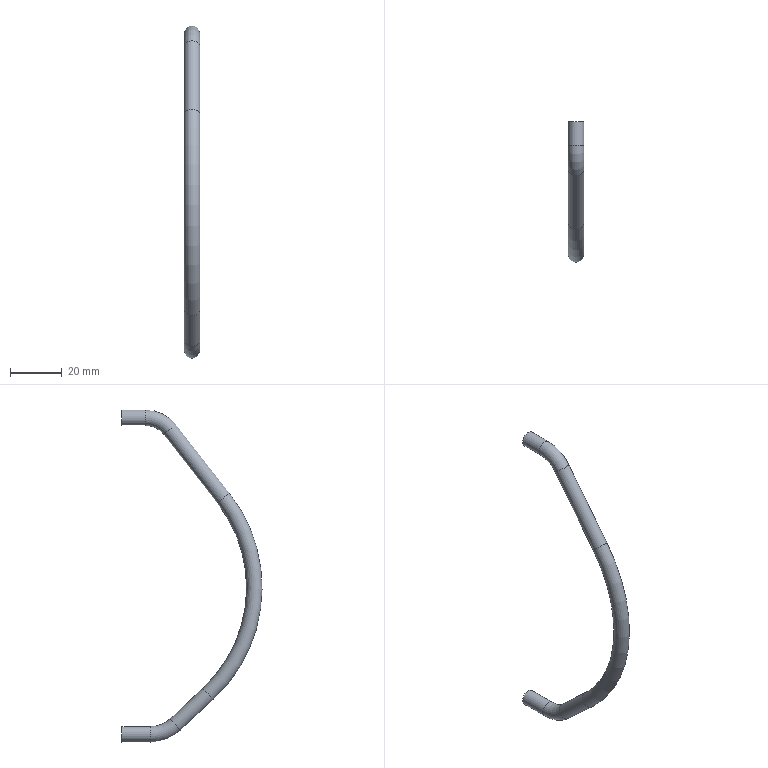Part | STEP file | 1-70.3 | 1 solid | 16 faces | box 6 x 54 x 128 mm | volume 1514 mm3 | cylinder 8 | torus 6 | plane 2 | commonest cylinder face diameters 5 x4 6 x4
STEP:
#1=CARTESIAN_POINT('',(0.,0.,0.));
#2=DIRECTION('',(0.,0.,1.));
#3=DIRECTION('',(1.,0.,0.));
#4=AXIS2_PLACEMENT_3D('',#1,#2,#3);
#5=CARTESIAN_POINT('',(-3.,0.,0.));
#6=VERTEX_POINT('',#5);
#7=CARTESIAN_POINT('',(0.,0.,0.));
#8=DIRECTION('',(0.,1.,0.));
#9=DIRECTION('',(-1.,0.,0.));
#10=AXIS2_PLACEMENT_3D('',#7,#8,#9);
#11=CIRCLE('',#10,3.);
#12=CARTESIAN_POINT('',(0.,0.,0.));
#13=DIRECTION('',(0.,-1.,0.));
#14=DIRECTION('',(-1.,0.,0.));
#15=AXIS2_PLACEMENT_3D('',#12,#13,#14);
#16=CYLINDRICAL_SURFACE('',#15,3.);
#17=CARTESIAN_POINT('',(6.283,0.));
#18=DIRECTION('',(-1.,0.));
#19=VECTOR('',#18,1.);
#20=LINE('',#17,#19);
#21=(GEOMETRIC_REPRESENTATION_CONTEXT(2)PARAMETRIC_REPRESENTATION_CONTEXT()REPRESENTATION_CONTEXT('',''));
#22=DEFINITIONAL_REPRESENTATION('',(#20),#21);
#23=PCURVE('',#16,#22);
#24=CARTESIAN_POINT('',(0.,0.,0.));
#25=DIRECTION('',(0.,1.,0.));
#26=DIRECTION('',(1.,0.,0.));
#27=AXIS2_PLACEMENT_3D('',#24,#25,#26);
#28=PLANE('',#27);
#29=CARTESIAN_POINT('',(0.,0.));
#30=DIRECTION('',(-1.,0.));
#31=AXIS2_PLACEMENT_2D('',#29,#30);
#32=CIRCLE('',#31,3.);
#33=(GEOMETRIC_REPRESENTATION_CONTEXT(2)PARAMETRIC_REPRESENTATION_CONTEXT()REPRESENTATION_CONTEXT('',''));
#34=DEFINITIONAL_REPRESENTATION('',(#32),#33);
#35=PCURVE('',#28,#34);
#36=SURFACE_CURVE('',#11,(#23,#35),.PCURVE_S1.);
#37=EDGE_CURVE('',#6,#6,#36,.T.);
#38=ORIENTED_EDGE('',*,*,#37,.F.);
#39=CARTESIAN_POINT('',(-3.,-9.,0.));
#40=VERTEX_POINT('',#39);
#41=CARTESIAN_POINT('',(-3.,0.,0.));
#42=DIRECTION('',(0.,-1.,0.));
#43=VECTOR('',#42,1.);
#44=LINE('',#41,#43);
#45=CARTESIAN_POINT('',(6.283,0.));
#46=DIRECTION('',(0.,1.));
#47=VECTOR('',#46,1.);
#48=LINE('',#45,#47);
#49=(GEOMETRIC_REPRESENTATION_CONTEXT(2)PARAMETRIC_REPRESENTATION_CONTEXT()REPRESENTATION_CONTEXT('',''));
#50=DEFINITIONAL_REPRESENTATION('',(#48),#49);
#51=PCURVE('',#16,#50);
#52=CARTESIAN_POINT('',(0.,0.));
#53=DIRECTION('',(0.,1.));
#54=VECTOR('',#53,1.);
#55=LINE('',#52,#54);
#56=(GEOMETRIC_REPRESENTATION_CONTEXT(2)PARAMETRIC_REPRESENTATION_CONTEXT()REPRESENTATION_CONTEXT('',''));
#57=DEFINITIONAL_REPRESENTATION('',(#55),#56);
#58=PCURVE('',#16,#57);
#59=SEAM_CURVE('',#44,(#51,#58),.PCURVE_S1.);
#60=EDGE_CURVE('',#6,#40,#59,.T.);
#61=ORIENTED_EDGE('',*,*,#60,.T.);
#62=CARTESIAN_POINT('',(0.,-9.,0.));
#63=DIRECTION('',(0.,-1.,0.));
#64=DIRECTION('',(-1.,0.,0.));
#65=AXIS2_PLACEMENT_3D('',#62,#63,#64);
#66=CIRCLE('',#65,3.);
#67=CARTESIAN_POINT('',(0.,9.));
#68=DIRECTION('',(1.,0.));
#69=VECTOR('',#68,1.);
#70=LINE('',#67,#69);
#71=(GEOMETRIC_REPRESENTATION_CONTEXT(2)PARAMETRIC_REPRESENTATION_CONTEXT()REPRESENTATION_CONTEXT('',''));
#72=DEFINITIONAL_REPRESENTATION('',(#70),#71);
#73=PCURVE('',#16,#72);
#74=CARTESIAN_POINT('',(0.,-9.,-12.));
#75=DIRECTION('',(-1.,0.,0.));
#76=DIRECTION('',(0.,0.,1.));
#77=AXIS2_PLACEMENT_3D('',#74,#75,#76);
#78=TOROIDAL_SURFACE('',#77,12.,3.);
#79=CARTESIAN_POINT('',(6.283,1.571));
#80=DIRECTION('',(0.,1.));
#81=VECTOR('',#80,1.);
#82=LINE('',#79,#81);
#83=(GEOMETRIC_REPRESENTATION_CONTEXT(2)PARAMETRIC_REPRESENTATION_CONTEXT()REPRESENTATION_CONTEXT('',''));
#84=DEFINITIONAL_REPRESENTATION('',(#82),#83);
#85=PCURVE('',#78,#84);
#86=SURFACE_CURVE('',#66,(#73,#85),.PCURVE_S1.);
#87=EDGE_CURVE('',#40,#40,#86,.T.);
#88=ORIENTED_EDGE('',*,*,#87,.F.);
#89=ORIENTED_EDGE('',*,*,#60,.F.);
#90=EDGE_LOOP('',(#38,#61,#88,#89));
#91=FACE_BOUND('',#90,.T.);
#92=ADVANCED_FACE('',(#91),#16,.T.);
#93=ORIENTED_EDGE('',*,*,#87,.T.);
#94=CARTESIAN_POINT('',(-3.,-18.45,-4.604));
#95=VERTEX_POINT('',#94);
#96=CARTESIAN_POINT('',(-3.,-9.,-12.));
#97=DIRECTION('',(1.,0.,0.));
#98=DIRECTION('',(0.,0.,1.));
#99=AXIS2_PLACEMENT_3D('',#96,#97,#98);
#100=CIRCLE('',#99,12.);
#101=CARTESIAN_POINT('',(6.283,7.854));
#102=DIRECTION('',(-1.,0.));
#103=VECTOR('',#102,1.);
#104=LINE('',#101,#103);
#105=(GEOMETRIC_REPRESENTATION_CONTEXT(2)PARAMETRIC_REPRESENTATION_CONTEXT()REPRESENTATION_CONTEXT('',''));
#106=DEFINITIONAL_REPRESENTATION('',(#104),#105);
#107=PCURVE('',#78,#106);
#108=CARTESIAN_POINT('',(6.283,1.571));
#109=DIRECTION('',(-1.,0.));
#110=VECTOR('',#109,1.);
#111=LINE('',#108,#110);
#112=(GEOMETRIC_REPRESENTATION_CONTEXT(2)PARAMETRIC_REPRESENTATION_CONTEXT()REPRESENTATION_CONTEXT('',''));
#113=DEFINITIONAL_REPRESENTATION('',(#111),#112);
#114=PCURVE('',#78,#113);
#115=SEAM_CURVE('',#100,(#107,#114),.PCURVE_S1.);
#116=EDGE_CURVE('',#40,#95,#115,.T.);
#117=ORIENTED_EDGE('',*,*,#116,.T.);
#118=CARTESIAN_POINT('',(0.,-18.45,-4.604));
#119=DIRECTION('',(0.,0.6164,0.7875));
#120=DIRECTION('',(-1.,0.,0.));
#121=AXIS2_PLACEMENT_3D('',#118,#119,#120);
#122=CIRCLE('',#121,3.);
#123=CARTESIAN_POINT('',(5.377,7.854));
#124=DIRECTION('',(0.,-1.));
#125=VECTOR('',#124,1.);
#126=LINE('',#123,#125);
#127=(GEOMETRIC_REPRESENTATION_CONTEXT(2)PARAMETRIC_REPRESENTATION_CONTEXT()REPRESENTATION_CONTEXT('',''));
#128=DEFINITIONAL_REPRESENTATION('',(#126),#127);
#129=PCURVE('',#78,#128);
#130=CARTESIAN_POINT('',(0.,-18.45,-4.604));
#131=DIRECTION('',(0.,-0.6164,-0.7875));
#132=DIRECTION('',(-1.,0.,0.));
#133=AXIS2_PLACEMENT_3D('',#130,#131,#132);
#134=CYLINDRICAL_SURFACE('',#133,3.);
#135=CARTESIAN_POINT('',(6.283,0.));
#136=DIRECTION('',(-1.,0.));
#137=VECTOR('',#136,1.);
#138=LINE('',#135,#137);
#139=(GEOMETRIC_REPRESENTATION_CONTEXT(2)PARAMETRIC_REPRESENTATION_CONTEXT()REPRESENTATION_CONTEXT('',''));
#140=DEFINITIONAL_REPRESENTATION('',(#138),#139);
#141=PCURVE('',#134,#140);
#142=SURFACE_CURVE('',#122,(#129,#141),.PCURVE_S1.);
#143=EDGE_CURVE('',#95,#95,#142,.T.);
#144=ORIENTED_EDGE('',*,*,#143,.T.);
#145=ORIENTED_EDGE('',*,*,#116,.F.);
#146=EDGE_LOOP('',(#93,#117,#144,#145));
#147=FACE_BOUND('',#146,.T.);
#148=ADVANCED_FACE('',(#147),#78,.T.);
#149=ORIENTED_EDGE('',*,*,#143,.F.);
#150=CARTESIAN_POINT('',(-3.,-39.098,-30.984));
#151=VERTEX_POINT('',#150);
#152=CARTESIAN_POINT('',(-3.,-18.45,-4.604));
#153=DIRECTION('',(0.,-0.6164,-0.7875));
#154=VECTOR('',#153,1.);
#155=LINE('',#152,#154);
#156=CARTESIAN_POINT('',(6.283,0.));
#157=DIRECTION('',(0.,1.));
#158=VECTOR('',#157,1.);
#159=LINE('',#156,#158);
#160=(GEOMETRIC_REPRESENTATION_CONTEXT(2)PARAMETRIC_REPRESENTATION_CONTEXT()REPRESENTATION_CONTEXT('',''));
#161=DEFINITIONAL_REPRESENTATION('',(#159),#160);
#162=PCURVE('',#134,#161);
#163=CARTESIAN_POINT('',(0.,0.));
#164=DIRECTION('',(0.,1.));
#165=VECTOR('',#164,1.);
#166=LINE('',#163,#165);
#167=(GEOMETRIC_REPRESENTATION_CONTEXT(2)PARAMETRIC_REPRESENTATION_CONTEXT()REPRESENTATION_CONTEXT('',''));
#168=DEFINITIONAL_REPRESENTATION('',(#166),#167);
#169=PCURVE('',#134,#168);
#170=SEAM_CURVE('',#155,(#162,#169),.PCURVE_S1.);
#171=EDGE_CURVE('',#95,#151,#170,.T.);
#172=ORIENTED_EDGE('',*,*,#171,.T.);
#173=CARTESIAN_POINT('',(0.,-39.098,-30.984));
#174=DIRECTION('',(0.,-0.6164,-0.7875));
#175=DIRECTION('',(-1.,0.,0.));
#176=AXIS2_PLACEMENT_3D('',#173,#174,#175);
#177=CIRCLE('',#176,3.);
#178=CARTESIAN_POINT('',(0.,33.5));
#179=DIRECTION('',(1.,0.));
#180=VECTOR('',#179,1.);
#181=LINE('',#178,#180);
#182=(GEOMETRIC_REPRESENTATION_CONTEXT(2)PARAMETRIC_REPRESENTATION_CONTEXT()REPRESENTATION_CONTEXT('',''));
#183=DEFINITIONAL_REPRESENTATION('',(#181),#182);
#184=PCURVE('',#134,#183);
#185=CARTESIAN_POINT('',(0.,5.,-65.5));
#186=DIRECTION('',(-1.,0.,0.));
#187=DIRECTION('',(0.,-0.7875,0.6164));
#188=AXIS2_PLACEMENT_3D('',#185,#186,#187);
#189=TOROIDAL_SURFACE('',#188,56.,3.);
#190=CARTESIAN_POINT('',(6.283,1.571));
#191=DIRECTION('',(0.,1.));
#192=VECTOR('',#191,1.);
#193=LINE('',#190,#192);
#194=(GEOMETRIC_REPRESENTATION_CONTEXT(2)PARAMETRIC_REPRESENTATION_CONTEXT()REPRESENTATION_CONTEXT('',''));
#195=DEFINITIONAL_REPRESENTATION('',(#193),#194);
#196=PCURVE('',#189,#195);
#197=SURFACE_CURVE('',#177,(#184,#196),.PCURVE_S1.);
#198=EDGE_CURVE('',#151,#151,#197,.T.);
#199=ORIENTED_EDGE('',*,*,#198,.F.);
#200=ORIENTED_EDGE('',*,*,#171,.F.);
#201=EDGE_LOOP('',(#149,#172,#199,#200));
#202=FACE_BOUND('',#201,.T.);
#203=ADVANCED_FACE('',(#202),#134,.T.);
#204=ORIENTED_EDGE('',*,*,#198,.T.);
#205=CARTESIAN_POINT('',(-3.,-33.179,-106.468));
#206=VERTEX_POINT('',#205);
#207=CARTESIAN_POINT('',(-3.,5.,-65.5));
#208=DIRECTION('',(1.,0.,0.));
#209=DIRECTION('',(0.,-0.7875,0.6164));
#210=AXIS2_PLACEMENT_3D('',#207,#208,#209);
#211=CIRCLE('',#210,56.);
#212=CARTESIAN_POINT('',(6.283,7.854));
#213=DIRECTION('',(-1.,0.));
#214=VECTOR('',#213,1.);
#215=LINE('',#212,#214);
#216=(GEOMETRIC_REPRESENTATION_CONTEXT(2)PARAMETRIC_REPRESENTATION_CONTEXT()REPRESENTATION_CONTEXT('',''));
#217=DEFINITIONAL_REPRESENTATION('',(#215),#216);
#218=PCURVE('',#189,#217);
#219=CARTESIAN_POINT('',(6.283,1.571));
#220=DIRECTION('',(-1.,0.));
#221=VECTOR('',#220,1.);
#222=LINE('',#219,#221);
#223=(GEOMETRIC_REPRESENTATION_CONTEXT(2)PARAMETRIC_REPRESENTATION_CONTEXT()REPRESENTATION_CONTEXT('',''));
#224=DEFINITIONAL_REPRESENTATION('',(#222),#223);
#225=PCURVE('',#189,#224);
#226=SEAM_CURVE('',#211,(#218,#225),.PCURVE_S1.);
#227=EDGE_CURVE('',#151,#206,#226,.T.);
#228=ORIENTED_EDGE('',*,*,#227,.T.);
#229=CARTESIAN_POINT('',(3.,-33.179,-106.468));
#230=VERTEX_POINT('',#229);
#231=CARTESIAN_POINT('',(0.,-33.179,-106.468));
#232=DIRECTION('',(0.,-0.7316,0.6818));
#233=DIRECTION('',(-1.,0.,0.));
#234=AXIS2_PLACEMENT_3D('',#231,#232,#233);
#235=CIRCLE('',#234,3.);
#236=CARTESIAN_POINT('',(4.798,7.854));
#237=DIRECTION('',(0.,-1.));
#238=VECTOR('',#237,1.);
#239=LINE('',#236,#238);
#240=(GEOMETRIC_REPRESENTATION_CONTEXT(2)PARAMETRIC_REPRESENTATION_CONTEXT()REPRESENTATION_CONTEXT('',''));
#241=DEFINITIONAL_REPRESENTATION('',(#239),#240);
#242=PCURVE('',#189,#241);
#243=CARTESIAN_POINT('',(0.,-33.179,-106.468));
#244=DIRECTION('',(0.,0.7316,-0.6818));
#245=DIRECTION('',(1.,0.,0.));
#246=AXIS2_PLACEMENT_3D('',#243,#244,#245);
#247=CYLINDRICAL_SURFACE('',#246,3.);
#248=CARTESIAN_POINT('',(3.142,0.));
#249=DIRECTION('',(-1.,0.));
#250=VECTOR('',#249,1.);
#251=LINE('',#248,#250);
#252=(GEOMETRIC_REPRESENTATION_CONTEXT(2)PARAMETRIC_REPRESENTATION_CONTEXT()REPRESENTATION_CONTEXT('',''));
#253=DEFINITIONAL_REPRESENTATION('',(#251),#252);
#254=PCURVE('',#247,#253);
#255=SURFACE_CURVE('',#235,(#242,#254),.PCURVE_S1.);
#256=EDGE_CURVE('',#206,#230,#255,.T.);
#257=ORIENTED_EDGE('',*,*,#256,.T.);
#258=CARTESIAN_POINT('',(0.,-33.179,-106.468));
#259=DIRECTION('',(0.,-0.7316,0.6818));
#260=DIRECTION('',(1.,0.,0.));
#261=AXIS2_PLACEMENT_3D('',#258,#259,#260);
#262=CIRCLE('',#261,3.);
#263=CARTESIAN_POINT('',(4.798,4.712));
#264=DIRECTION('',(0.,-1.));
#265=VECTOR('',#264,1.);
#266=LINE('',#263,#265);
#267=(GEOMETRIC_REPRESENTATION_CONTEXT(2)PARAMETRIC_REPRESENTATION_CONTEXT()REPRESENTATION_CONTEXT('',''));
#268=DEFINITIONAL_REPRESENTATION('',(#266),#267);
#269=PCURVE('',#189,#268);
#270=CARTESIAN_POINT('',(6.283,0.));
#271=DIRECTION('',(-1.,0.));
#272=VECTOR('',#271,1.);
#273=LINE('',#270,#272);
#274=(GEOMETRIC_REPRESENTATION_CONTEXT(2)PARAMETRIC_REPRESENTATION_CONTEXT()REPRESENTATION_CONTEXT('',''));
#275=DEFINITIONAL_REPRESENTATION('',(#273),#274);
#276=PCURVE('',#247,#275);
#277=SURFACE_CURVE('',#262,(#269,#276),.PCURVE_S1.);
#278=EDGE_CURVE('',#230,#206,#277,.T.);
#279=ORIENTED_EDGE('',*,*,#278,.T.);
#280=ORIENTED_EDGE('',*,*,#227,.F.);
#281=EDGE_LOOP('',(#204,#228,#257,#279,#280));
#282=FACE_BOUND('',#281,.T.);
#283=ADVANCED_FACE('',(#282),#189,.T.);
#284=ORIENTED_EDGE('',*,*,#256,.F.);
#285=ORIENTED_EDGE('',*,*,#278,.F.);
#286=CARTESIAN_POINT('',(3.,-20.545,-118.242));
#287=VERTEX_POINT('',#286);
#288=CARTESIAN_POINT('',(3.,-33.179,-106.468));
#289=DIRECTION('',(0.,0.7316,-0.6818));
#290=VECTOR('',#289,1.);
#291=LINE('',#288,#290);
#292=CARTESIAN_POINT('',(6.283,0.));
#293=DIRECTION('',(0.,1.));
#294=VECTOR('',#293,1.);
#295=LINE('',#292,#294);
#296=(GEOMETRIC_REPRESENTATION_CONTEXT(2)PARAMETRIC_REPRESENTATION_CONTEXT()REPRESENTATION_CONTEXT('',''));
#297=DEFINITIONAL_REPRESENTATION('',(#295),#296);
#298=PCURVE('',#247,#297);
#299=CARTESIAN_POINT('',(0.,0.));
#300=DIRECTION('',(0.,1.));
#301=VECTOR('',#300,1.);
#302=LINE('',#299,#301);
#303=(GEOMETRIC_REPRESENTATION_CONTEXT(2)PARAMETRIC_REPRESENTATION_CONTEXT()REPRESENTATION_CONTEXT('',''));
#304=DEFINITIONAL_REPRESENTATION('',(#302),#303);
#305=PCURVE('',#247,#304);
#306=SEAM_CURVE('',#291,(#298,#305),.PCURVE_S1.);
#307=EDGE_CURVE('',#230,#287,#306,.T.);
#308=ORIENTED_EDGE('',*,*,#307,.T.);
#309=CARTESIAN_POINT('',(-3.,-20.545,-118.242));
#310=VERTEX_POINT('',#309);
#311=CARTESIAN_POINT('',(0.,-20.545,-118.242));
#312=DIRECTION('',(0.,0.7316,-0.6818));
#313=DIRECTION('',(-1.,0.,0.));
#314=AXIS2_PLACEMENT_3D('',#311,#312,#313);
#315=CIRCLE('',#314,3.);
#316=CARTESIAN_POINT('',(3.142,17.27));
#317=DIRECTION('',(1.,0.));
#318=VECTOR('',#317,1.);
#319=LINE('',#316,#318);
#320=(GEOMETRIC_REPRESENTATION_CONTEXT(2)PARAMETRIC_REPRESENTATION_CONTEXT()REPRESENTATION_CONTEXT('',''));
#321=DEFINITIONAL_REPRESENTATION('',(#319),#320);
#322=PCURVE('',#247,#321);
#323=CARTESIAN_POINT('',(0.,-11.,-108.));
#324=DIRECTION('',(-1.,0.,0.));
#325=DIRECTION('',(0.,-0.6818,-0.7316));
#326=AXIS2_PLACEMENT_3D('',#323,#324,#325);
#327=TOROIDAL_SURFACE('',#326,14.,3.);
#328=CARTESIAN_POINT('',(6.283,1.571));
#329=DIRECTION('',(0.,1.));
#330=VECTOR('',#329,1.);
#331=LINE('',#328,#330);
#332=(GEOMETRIC_REPRESENTATION_CONTEXT(2)PARAMETRIC_REPRESENTATION_CONTEXT()REPRESENTATION_CONTEXT('',''));
#333=DEFINITIONAL_REPRESENTATION('',(#331),#332);
#334=PCURVE('',#327,#333);
#335=SURFACE_CURVE('',#315,(#322,#334),.PCURVE_S1.);
#336=EDGE_CURVE('',#310,#287,#335,.T.);
#337=ORIENTED_EDGE('',*,*,#336,.F.);
#338=CARTESIAN_POINT('',(0.,-20.545,-118.242));
#339=DIRECTION('',(0.,0.7316,-0.6818));
#340=DIRECTION('',(1.,0.,0.));
#341=AXIS2_PLACEMENT_3D('',#338,#339,#340);
#342=CIRCLE('',#341,3.);
#343=CARTESIAN_POINT('',(0.,17.27));
#344=DIRECTION('',(1.,0.));
#345=VECTOR('',#344,1.);
#346=LINE('',#343,#345);
#347=(GEOMETRIC_REPRESENTATION_CONTEXT(2)PARAMETRIC_REPRESENTATION_CONTEXT()REPRESENTATION_CONTEXT('',''));
#348=DEFINITIONAL_REPRESENTATION('',(#346),#347);
#349=PCURVE('',#247,#348);
#350=CARTESIAN_POINT('',(6.283,4.712));
#351=DIRECTION('',(0.,1.));
#352=VECTOR('',#351,1.);
#353=LINE('',#350,#352);
#354=(GEOMETRIC_REPRESENTATION_CONTEXT(2)PARAMETRIC_REPRESENTATION_CONTEXT()REPRESENTATION_CONTEXT('',''));
#355=DEFINITIONAL_REPRESENTATION('',(#353),#354);
#356=PCURVE('',#327,#355);
#357=SURFACE_CURVE('',#342,(#349,#356),.PCURVE_S1.);
#358=EDGE_CURVE('',#287,#310,#357,.T.);
#359=ORIENTED_EDGE('',*,*,#358,.F.);
#360=ORIENTED_EDGE('',*,*,#307,.F.);
#361=EDGE_LOOP('',(#284,#285,#308,#337,#359,#360));
#362=FACE_BOUND('',#361,.T.);
#363=ADVANCED_FACE('',(#362),#247,.T.);
#364=ORIENTED_EDGE('',*,*,#336,.T.);
#365=ORIENTED_EDGE('',*,*,#358,.T.);
#366=CARTESIAN_POINT('',(-3.,-11.,-122.));
#367=VERTEX_POINT('',#366);
#368=CARTESIAN_POINT('',(-3.,-11.,-108.));
#369=DIRECTION('',(1.,0.,0.));
#370=DIRECTION('',(0.,-0.6818,-0.7316));
#371=AXIS2_PLACEMENT_3D('',#368,#369,#370);
#372=CIRCLE('',#371,14.);
#373=CARTESIAN_POINT('',(6.283,7.854));
#374=DIRECTION('',(-1.,0.));
#375=VECTOR('',#374,1.);
#376=LINE('',#373,#375);
#377=(GEOMETRIC_REPRESENTATION_CONTEXT(2)PARAMETRIC_REPRESENTATION_CONTEXT()REPRESENTATION_CONTEXT('',''));
#378=DEFINITIONAL_REPRESENTATION('',(#376),#377);
#379=PCURVE('',#327,#378);
#380=CARTESIAN_POINT('',(6.283,1.571));
#381=DIRECTION('',(-1.,0.));
#382=VECTOR('',#381,1.);
#383=LINE('',#380,#382);
#384=(GEOMETRIC_REPRESENTATION_CONTEXT(2)PARAMETRIC_REPRESENTATION_CONTEXT()REPRESENTATION_CONTEXT('',''));
#385=DEFINITIONAL_REPRESENTATION('',(#383),#384);
#386=PCURVE('',#327,#385);
#387=SEAM_CURVE('',#372,(#379,#386),.PCURVE_S1.);
#388=EDGE_CURVE('',#310,#367,#387,.T.);
#389=ORIENTED_EDGE('',*,*,#388,.T.);
#390=CARTESIAN_POINT('',(3.,-11.,-122.));
#391=VERTEX_POINT('',#390);
#392=CARTESIAN_POINT('',(0.,-11.,-122.));
#393=DIRECTION('',(0.,-1.,0.));
#394=DIRECTION('',(-1.,0.,0.));
#395=AXIS2_PLACEMENT_3D('',#392,#393,#394);
#396=CIRCLE('',#395,3.);
#397=CARTESIAN_POINT('',(5.533,7.854));
#398=DIRECTION('',(0.,-1.));
#399=VECTOR('',#398,1.);
#400=LINE('',#397,#399);
#401=(GEOMETRIC_REPRESENTATION_CONTEXT(2)PARAMETRIC_REPRESENTATION_CONTEXT()REPRESENTATION_CONTEXT('',''));
#402=DEFINITIONAL_REPRESENTATION('',(#400),#401);
#403=PCURVE('',#327,#402);
#404=CARTESIAN_POINT('',(0.,-11.,-122.));
#405=DIRECTION('',(0.,1.,0.));
#406=DIRECTION('',(1.,0.,0.));
#407=AXIS2_PLACEMENT_3D('',#404,#405,#406);
#408=CYLINDRICAL_SURFACE('',#407,3.);
#409=CARTESIAN_POINT('',(3.142,0.));
#410=DIRECTION('',(-1.,0.));
#411=VECTOR('',#410,1.);
#412=LINE('',#409,#411);
#413=(GEOMETRIC_REPRESENTATION_CONTEXT(2)PARAMETRIC_REPRESENTATION_CONTEXT()REPRESENTATION_CONTEXT('',''));
#414=DEFINITIONAL_REPRESENTATION('',(#412),#413);
#415=PCURVE('',#408,#414);
#416=SURFACE_CURVE('',#396,(#403,#415),.PCURVE_S1.);
#417=EDGE_CURVE('',#367,#391,#416,.T.);
#418=ORIENTED_EDGE('',*,*,#417,.T.);
#419=CARTESIAN_POINT('',(0.,-11.,-122.));
#420=DIRECTION('',(0.,-1.,0.));
#421=DIRECTION('',(1.,0.,0.));
#422=AXIS2_PLACEMENT_3D('',#419,#420,#421);
#423=CIRCLE('',#422,3.);
#424=CARTESIAN_POINT('',(5.533,4.712));
#425=DIRECTION('',(0.,-1.));
#426=VECTOR('',#425,1.);
#427=LINE('',#424,#426);
#428=(GEOMETRIC_REPRESENTATION_CONTEXT(2)PARAMETRIC_REPRESENTATION_CONTEXT()REPRESENTATION_CONTEXT('',''));
#429=DEFINITIONAL_REPRESENTATION('',(#427),#428);
#430=PCURVE('',#327,#429);
#431=CARTESIAN_POINT('',(6.283,0.));
#432=DIRECTION('',(-1.,0.));
#433=VECTOR('',#432,1.);
#434=LINE('',#431,#433);
#435=(GEOMETRIC_REPRESENTATION_CONTEXT(2)PARAMETRIC_REPRESENTATION_CONTEXT()REPRESENTATION_CONTEXT('',''));
#436=DEFINITIONAL_REPRESENTATION('',(#434),#435);
#437=PCURVE('',#408,#436);
#438=SURFACE_CURVE('',#423,(#430,#437),.PCURVE_S1.);
#439=EDGE_CURVE('',#391,#367,#438,.T.);
#440=ORIENTED_EDGE('',*,*,#439,.T.);
#441=ORIENTED_EDGE('',*,*,#388,.F.);
#442=EDGE_LOOP('',(#364,#365,#389,#418,#440,#441));
#443=FACE_BOUND('',#442,.T.);
#444=ADVANCED_FACE('',(#443),#327,.T.);
#445=ORIENTED_EDGE('',*,*,#417,.F.);
#446=ORIENTED_EDGE('',*,*,#439,.F.);
#447=CARTESIAN_POINT('',(3.,0.,-122.));
#448=VERTEX_POINT('',#447);
#449=CARTESIAN_POINT('',(3.,-11.,-122.));
#450=DIRECTION('',(0.,1.,0.));
#451=VECTOR('',#450,1.);
#452=LINE('',#449,#451);
#453=CARTESIAN_POINT('',(6.283,0.));
#454=DIRECTION('',(0.,1.));
#455=VECTOR('',#454,1.);
#456=LINE('',#453,#455);
#457=(GEOMETRIC_REPRESENTATION_CONTEXT(2)PARAMETRIC_REPRESENTATION_CONTEXT()REPRESENTATION_CONTEXT('',''));
#458=DEFINITIONAL_REPRESENTATION('',(#456),#457);
#459=PCURVE('',#408,#458);
#460=CARTESIAN_POINT('',(0.,0.));
#461=DIRECTION('',(0.,1.));
#462=VECTOR('',#461,1.);
#463=LINE('',#460,#462);
#464=(GEOMETRIC_REPRESENTATION_CONTEXT(2)PARAMETRIC_REPRESENTATION_CONTEXT()REPRESENTATION_CONTEXT('',''));
#465=DEFINITIONAL_REPRESENTATION('',(#463),#464);
#466=PCURVE('',#408,#465);
#467=SEAM_CURVE('',#452,(#459,#466),.PCURVE_S1.);
#468=EDGE_CURVE('',#391,#448,#467,.T.);
#469=ORIENTED_EDGE('',*,*,#468,.T.);
#470=CARTESIAN_POINT('',(0.,0.,-122.));
#471=DIRECTION('',(0.,1.,0.));
#472=DIRECTION('',(1.,0.,0.));
#473=AXIS2_PLACEMENT_3D('',#470,#471,#472);
#474=CIRCLE('',#473,3.);
#475=CARTESIAN_POINT('',(0.,11.));
#476=DIRECTION('',(1.,0.));
#477=VECTOR('',#476,1.);
#478=LINE('',#475,#477);
#479=(GEOMETRIC_REPRESENTATION_CONTEXT(2)PARAMETRIC_REPRESENTATION_CONTEXT()REPRESENTATION_CONTEXT('',''));
#480=DEFINITIONAL_REPRESENTATION('',(#478),#479);
#481=PCURVE('',#408,#480);
#482=CARTESIAN_POINT('',(0.,0.,-122.));
#483=DIRECTION('',(0.,1.,0.));
#484=DIRECTION('',(0.,0.,1.));
#485=AXIS2_PLACEMENT_3D('',#482,#483,#484);
#486=PLANE('',#485);
#487=CARTESIAN_POINT('',(0.,0.));
#488=DIRECTION('',(0.,1.));
#489=AXIS2_PLACEMENT_2D('',#487,#488);
#490=CIRCLE('',#489,3.);
#491=(GEOMETRIC_REPRESENTATION_CONTEXT(2)PARAMETRIC_REPRESENTATION_CONTEXT()REPRESENTATION_CONTEXT('',''));
#492=DEFINITIONAL_REPRESENTATION('',(#490),#491);
#493=PCURVE('',#486,#492);
#494=SURFACE_CURVE('',#474,(#481,#493),.PCURVE_S1.);
#495=EDGE_CURVE('',#448,#448,#494,.T.);
#496=ORIENTED_EDGE('',*,*,#495,.F.);
#497=ORIENTED_EDGE('',*,*,#468,.F.);
#498=EDGE_LOOP('',(#445,#446,#469,#496,#497));
#499=FACE_BOUND('',#498,.T.);
#500=ADVANCED_FACE('',(#499),#408,.T.);
#501=ORIENTED_EDGE('',*,*,#37,.T.);
#502=EDGE_LOOP('',(#501));
#503=FACE_BOUND('',#502,.T.);
#504=CARTESIAN_POINT('',(-2.5,0.,0.));
#505=VERTEX_POINT('',#504);
#506=CARTESIAN_POINT('',(0.,0.,0.));
#507=DIRECTION('',(0.,1.,0.));
#508=DIRECTION('',(-1.,0.,0.));
#509=AXIS2_PLACEMENT_3D('',#506,#507,#508);
#510=CIRCLE('',#509,2.5);
#511=CARTESIAN_POINT('',(0.,0.));
#512=DIRECTION('',(-1.,0.));
#513=AXIS2_PLACEMENT_2D('',#511,#512);
#514=CIRCLE('',#513,2.5);
#515=(GEOMETRIC_REPRESENTATION_CONTEXT(2)PARAMETRIC_REPRESENTATION_CONTEXT()REPRESENTATION_CONTEXT('',''));
#516=DEFINITIONAL_REPRESENTATION('',(#514),#515);
#517=PCURVE('',#28,#516);
#518=CARTESIAN_POINT('',(0.,0.,0.));
#519=DIRECTION('',(0.,-1.,0.));
#520=DIRECTION('',(-1.,0.,0.));
#521=AXIS2_PLACEMENT_3D('',#518,#519,#520);
#522=CYLINDRICAL_SURFACE('',#521,2.5);
#523=CARTESIAN_POINT('',(6.283,0.));
#524=DIRECTION('',(-1.,0.));
#525=VECTOR('',#524,1.);
#526=LINE('',#523,#525);
#527=(GEOMETRIC_REPRESENTATION_CONTEXT(2)PARAMETRIC_REPRESENTATION_CONTEXT()REPRESENTATION_CONTEXT('',''));
#528=DEFINITIONAL_REPRESENTATION('',(#526),#527);
#529=PCURVE('',#522,#528);
#530=SURFACE_CURVE('',#510,(#517,#529),.PCURVE_S1.);
#531=EDGE_CURVE('',#505,#505,#530,.T.);
#532=ORIENTED_EDGE('',*,*,#531,.F.);
#533=EDGE_LOOP('',(#532));
#534=FACE_BOUND('',#533,.T.);
#535=ADVANCED_FACE('',(#503,#534),#28,.T.);
#536=ORIENTED_EDGE('',*,*,#495,.T.);
#537=EDGE_LOOP('',(#536));
#538=FACE_BOUND('',#537,.T.);
#539=CARTESIAN_POINT('',(2.5,0.,-122.));
#540=VERTEX_POINT('',#539);
#541=CARTESIAN_POINT('',(0.,0.,-122.));
#542=DIRECTION('',(0.,1.,0.));
#543=DIRECTION('',(1.,0.,0.));
#544=AXIS2_PLACEMENT_3D('',#541,#542,#543);
#545=CIRCLE('',#544,2.5);
#546=CARTESIAN_POINT('',(0.,0.));
#547=DIRECTION('',(0.,1.));
#548=AXIS2_PLACEMENT_2D('',#546,#547);
#549=CIRCLE('',#548,2.5);
#550=(GEOMETRIC_REPRESENTATION_CONTEXT(2)PARAMETRIC_REPRESENTATION_CONTEXT()REPRESENTATION_CONTEXT('',''));
#551=DEFINITIONAL_REPRESENTATION('',(#549),#550);
#552=PCURVE('',#486,#551);
#553=CARTESIAN_POINT('',(0.,-11.,-122.));
#554=DIRECTION('',(0.,1.,0.));
#555=DIRECTION('',(1.,0.,0.));
#556=AXIS2_PLACEMENT_3D('',#553,#554,#555);
#557=CYLINDRICAL_SURFACE('',#556,2.5);
#558=CARTESIAN_POINT('',(0.,11.));
#559=DIRECTION('',(1.,0.));
#560=VECTOR('',#559,1.);
#561=LINE('',#558,#560);
#562=(GEOMETRIC_REPRESENTATION_CONTEXT(2)PARAMETRIC_REPRESENTATION_CONTEXT()REPRESENTATION_CONTEXT('',''));
#563=DEFINITIONAL_REPRESENTATION('',(#561),#562);
#564=PCURVE('',#557,#563);
#565=SURFACE_CURVE('',#545,(#552,#564),.PCURVE_S1.);
#566=EDGE_CURVE('',#540,#540,#565,.T.);
#567=ORIENTED_EDGE('',*,*,#566,.F.);
#568=EDGE_LOOP('',(#567));
#569=FACE_BOUND('',#568,.T.);
#570=ADVANCED_FACE('',(#538,#569),#486,.T.);
#571=ORIENTED_EDGE('',*,*,#531,.F.);
#572=CARTESIAN_POINT('',(-2.5,-9.,0.));
#573=VERTEX_POINT('',#572);
#574=CARTESIAN_POINT('',(-2.5,0.,0.));
#575=DIRECTION('',(0.,-1.,0.));
#576=VECTOR('',#575,1.);
#577=LINE('',#574,#576);
#578=CARTESIAN_POINT('',(6.283,0.));
#579=DIRECTION('',(0.,1.));
#580=VECTOR('',#579,1.);
#581=LINE('',#578,#580);
#582=(GEOMETRIC_REPRESENTATION_CONTEXT(2)PARAMETRIC_REPRESENTATION_CONTEXT()REPRESENTATION_CONTEXT('',''));
#583=DEFINITIONAL_REPRESENTATION('',(#581),#582);
#584=PCURVE('',#522,#583);
#585=CARTESIAN_POINT('',(0.,0.));
#586=DIRECTION('',(0.,1.));
#587=VECTOR('',#586,1.);
#588=LINE('',#585,#587);
#589=(GEOMETRIC_REPRESENTATION_CONTEXT(2)PARAMETRIC_REPRESENTATION_CONTEXT()REPRESENTATION_CONTEXT('',''));
#590=DEFINITIONAL_REPRESENTATION('',(#588),#589);
#591=PCURVE('',#522,#590);
#592=SEAM_CURVE('',#577,(#584,#591),.PCURVE_S1.);
#593=EDGE_CURVE('',#505,#573,#592,.T.);
#594=ORIENTED_EDGE('',*,*,#593,.T.);
#595=CARTESIAN_POINT('',(0.,-9.,0.));
#596=DIRECTION('',(0.,-1.,0.));
#597=DIRECTION('',(-1.,0.,0.));
#598=AXIS2_PLACEMENT_3D('',#595,#596,#597);
#599=CIRCLE('',#598,2.5);
#600=CARTESIAN_POINT('',(0.,9.));
#601=DIRECTION('',(1.,0.));
#602=VECTOR('',#601,1.);
#603=LINE('',#600,#602);
#604=(GEOMETRIC_REPRESENTATION_CONTEXT(2)PARAMETRIC_REPRESENTATION_CONTEXT()REPRESENTATION_CONTEXT('',''));
#605=DEFINITIONAL_REPRESENTATION('',(#603),#604);
#606=PCURVE('',#522,#605);
#607=CARTESIAN_POINT('',(0.,-9.,-12.));
#608=DIRECTION('',(-1.,0.,0.));
#609=DIRECTION('',(0.,0.,1.));
#610=AXIS2_PLACEMENT_3D('',#607,#608,#609);
#611=TOROIDAL_SURFACE('',#610,12.,2.5);
#612=CARTESIAN_POINT('',(6.283,1.571));
#613=DIRECTION('',(0.,1.));
#614=VECTOR('',#613,1.);
#615=LINE('',#612,#614);
#616=(GEOMETRIC_REPRESENTATION_CONTEXT(2)PARAMETRIC_REPRESENTATION_CONTEXT()REPRESENTATION_CONTEXT('',''));
#617=DEFINITIONAL_REPRESENTATION('',(#615),#616);
#618=PCURVE('',#611,#617);
#619=SURFACE_CURVE('',#599,(#606,#618),.PCURVE_S1.);
#620=EDGE_CURVE('',#573,#573,#619,.T.);
#621=ORIENTED_EDGE('',*,*,#620,.F.);
#622=ORIENTED_EDGE('',*,*,#593,.F.);
#623=EDGE_LOOP('',(#571,#594,#621,#622));
#624=FACE_BOUND('',#623,.F.);
#625=ADVANCED_FACE('',(#624),#522,.F.);
#626=ORIENTED_EDGE('',*,*,#620,.T.);
#627=CARTESIAN_POINT('',(-2.5,-18.45,-4.604));
#628=VERTEX_POINT('',#627);
#629=CARTESIAN_POINT('',(-2.5,-9.,-12.));
#630=DIRECTION('',(1.,0.,0.));
#631=DIRECTION('',(0.,0.,1.));
#632=AXIS2_PLACEMENT_3D('',#629,#630,#631);
#633=CIRCLE('',#632,12.);
#634=CARTESIAN_POINT('',(6.283,7.854));
#635=DIRECTION('',(-1.,0.));
#636=VECTOR('',#635,1.);
#637=LINE('',#634,#636);
#638=(GEOMETRIC_REPRESENTATION_CONTEXT(2)PARAMETRIC_REPRESENTATION_CONTEXT()REPRESENTATION_CONTEXT('',''));
#639=DEFINITIONAL_REPRESENTATION('',(#637),#638);
#640=PCURVE('',#611,#639);
#641=CARTESIAN_POINT('',(6.283,1.571));
#642=DIRECTION('',(-1.,0.));
#643=VECTOR('',#642,1.);
#644=LINE('',#641,#643);
#645=(GEOMETRIC_REPRESENTATION_CONTEXT(2)PARAMETRIC_REPRESENTATION_CONTEXT()REPRESENTATION_CONTEXT('',''));
#646=DEFINITIONAL_REPRESENTATION('',(#644),#645);
#647=PCURVE('',#611,#646);
#648=SEAM_CURVE('',#633,(#640,#647),.PCURVE_S1.);
#649=EDGE_CURVE('',#573,#628,#648,.T.);
#650=ORIENTED_EDGE('',*,*,#649,.T.);
#651=CARTESIAN_POINT('',(0.,-18.45,-4.604));
#652=DIRECTION('',(0.,0.6164,0.7875));
#653=DIRECTION('',(-1.,0.,0.));
#654=AXIS2_PLACEMENT_3D('',#651,#652,#653);
#655=CIRCLE('',#654,2.5);
#656=CARTESIAN_POINT('',(5.377,7.854));
#657=DIRECTION('',(0.,-1.));
#658=VECTOR('',#657,1.);
#659=LINE('',#656,#658);
#660=(GEOMETRIC_REPRESENTATION_CONTEXT(2)PARAMETRIC_REPRESENTATION_CONTEXT()REPRESENTATION_CONTEXT('',''));
#661=DEFINITIONAL_REPRESENTATION('',(#659),#660);
#662=PCURVE('',#611,#661);
#663=CARTESIAN_POINT('',(0.,-18.45,-4.604));
#664=DIRECTION('',(0.,-0.6164,-0.7875));
#665=DIRECTION('',(-1.,0.,0.));
#666=AXIS2_PLACEMENT_3D('',#663,#664,#665);
#667=CYLINDRICAL_SURFACE('',#666,2.5);
#668=CARTESIAN_POINT('',(6.283,0.));
#669=DIRECTION('',(-1.,0.));
#670=VECTOR('',#669,1.);
#671=LINE('',#668,#670);
#672=(GEOMETRIC_REPRESENTATION_CONTEXT(2)PARAMETRIC_REPRESENTATION_CONTEXT()REPRESENTATION_CONTEXT('',''));
#673=DEFINITIONAL_REPRESENTATION('',(#671),#672);
#674=PCURVE('',#667,#673);
#675=SURFACE_CURVE('',#655,(#662,#674),.PCURVE_S1.);
#676=EDGE_CURVE('',#628,#628,#675,.T.);
#677=ORIENTED_EDGE('',*,*,#676,.T.);
#678=ORIENTED_EDGE('',*,*,#649,.F.);
#679=EDGE_LOOP('',(#626,#650,#677,#678));
#680=FACE_BOUND('',#679,.F.);
#681=ADVANCED_FACE('',(#680),#611,.F.);
#682=ORIENTED_EDGE('',*,*,#676,.F.);
#683=CARTESIAN_POINT('',(-2.5,-39.098,-30.984));
#684=VERTEX_POINT('',#683);
#685=CARTESIAN_POINT('',(-2.5,-18.45,-4.604));
#686=DIRECTION('',(0.,-0.6164,-0.7875));
#687=VECTOR('',#686,1.);
#688=LINE('',#685,#687);
#689=CARTESIAN_POINT('',(6.283,0.));
#690=DIRECTION('',(0.,1.));
#691=VECTOR('',#690,1.);
#692=LINE('',#689,#691);
#693=(GEOMETRIC_REPRESENTATION_CONTEXT(2)PARAMETRIC_REPRESENTATION_CONTEXT()REPRESENTATION_CONTEXT('',''));
#694=DEFINITIONAL_REPRESENTATION('',(#692),#693);
#695=PCURVE('',#667,#694);
#696=CARTESIAN_POINT('',(0.,0.));
#697=DIRECTION('',(0.,1.));
#698=VECTOR('',#697,1.);
#699=LINE('',#696,#698);
#700=(GEOMETRIC_REPRESENTATION_CONTEXT(2)PARAMETRIC_REPRESENTATION_CONTEXT()REPRESENTATION_CONTEXT('',''));
#701=DEFINITIONAL_REPRESENTATION('',(#699),#700);
#702=PCURVE('',#667,#701);
#703=SEAM_CURVE('',#688,(#695,#702),.PCURVE_S1.);
#704=EDGE_CURVE('',#628,#684,#703,.T.);
#705=ORIENTED_EDGE('',*,*,#704,.T.);
#706=CARTESIAN_POINT('',(0.,-39.098,-30.984));
#707=DIRECTION('',(0.,-0.6164,-0.7875));
#708=DIRECTION('',(-1.,0.,0.));
#709=AXIS2_PLACEMENT_3D('',#706,#707,#708);
#710=CIRCLE('',#709,2.5);
#711=CARTESIAN_POINT('',(0.,33.5));
#712=DIRECTION('',(1.,0.));
#713=VECTOR('',#712,1.);
#714=LINE('',#711,#713);
#715=(GEOMETRIC_REPRESENTATION_CONTEXT(2)PARAMETRIC_REPRESENTATION_CONTEXT()REPRESENTATION_CONTEXT('',''));
#716=DEFINITIONAL_REPRESENTATION('',(#714),#715);
#717=PCURVE('',#667,#716);
#718=CARTESIAN_POINT('',(0.,5.,-65.5));
#719=DIRECTION('',(-1.,0.,0.));
#720=DIRECTION('',(0.,-0.7875,0.6164));
#721=AXIS2_PLACEMENT_3D('',#718,#719,#720);
#722=TOROIDAL_SURFACE('',#721,56.,2.5);
#723=CARTESIAN_POINT('',(6.283,1.571));
#724=DIRECTION('',(0.,1.));
#725=VECTOR('',#724,1.);
#726=LINE('',#723,#725);
#727=(GEOMETRIC_REPRESENTATION_CONTEXT(2)PARAMETRIC_REPRESENTATION_CONTEXT()REPRESENTATION_CONTEXT('',''));
#728=DEFINITIONAL_REPRESENTATION('',(#726),#727);
#729=PCURVE('',#722,#728);
#730=SURFACE_CURVE('',#710,(#717,#729),.PCURVE_S1.);
#731=EDGE_CURVE('',#684,#684,#730,.T.);
#732=ORIENTED_EDGE('',*,*,#731,.F.);
#733=ORIENTED_EDGE('',*,*,#704,.F.);
#734=EDGE_LOOP('',(#682,#705,#732,#733));
#735=FACE_BOUND('',#734,.F.);
#736=ADVANCED_FACE('',(#735),#667,.F.);
#737=ORIENTED_EDGE('',*,*,#731,.T.);
#738=CARTESIAN_POINT('',(-2.5,-33.179,-106.468));
#739=VERTEX_POINT('',#738);
#740=CARTESIAN_POINT('',(-2.5,5.,-65.5));
#741=DIRECTION('',(1.,0.,0.));
#742=DIRECTION('',(0.,-0.7875,0.6164));
#743=AXIS2_PLACEMENT_3D('',#740,#741,#742);
#744=CIRCLE('',#743,56.);
#745=CARTESIAN_POINT('',(6.283,7.854));
#746=DIRECTION('',(-1.,0.));
#747=VECTOR('',#746,1.);
#748=LINE('',#745,#747);
#749=(GEOMETRIC_REPRESENTATION_CONTEXT(2)PARAMETRIC_REPRESENTATION_CONTEXT()REPRESENTATION_CONTEXT('',''));
#750=DEFINITIONAL_REPRESENTATION('',(#748),#749);
#751=PCURVE('',#722,#750);
#752=CARTESIAN_POINT('',(6.283,1.571));
#753=DIRECTION('',(-1.,0.));
#754=VECTOR('',#753,1.);
#755=LINE('',#752,#754);
#756=(GEOMETRIC_REPRESENTATION_CONTEXT(2)PARAMETRIC_REPRESENTATION_CONTEXT()REPRESENTATION_CONTEXT('',''));
#757=DEFINITIONAL_REPRESENTATION('',(#755),#756);
#758=PCURVE('',#722,#757);
#759=SEAM_CURVE('',#744,(#751,#758),.PCURVE_S1.);
#760=EDGE_CURVE('',#684,#739,#759,.T.);
#761=ORIENTED_EDGE('',*,*,#760,.T.);
#762=CARTESIAN_POINT('',(2.5,-33.179,-106.468));
#763=VERTEX_POINT('',#762);
#764=CARTESIAN_POINT('',(0.,-33.179,-106.468));
#765=DIRECTION('',(0.,-0.7316,0.6818));
#766=DIRECTION('',(-1.,0.,0.));
#767=AXIS2_PLACEMENT_3D('',#764,#765,#766);
#768=CIRCLE('',#767,2.5);
#769=CARTESIAN_POINT('',(4.798,7.854));
#770=DIRECTION('',(0.,-1.));
#771=VECTOR('',#770,1.);
#772=LINE('',#769,#771);
#773=(GEOMETRIC_REPRESENTATION_CONTEXT(2)PARAMETRIC_REPRESENTATION_CONTEXT()REPRESENTATION_CONTEXT('',''));
#774=DEFINITIONAL_REPRESENTATION('',(#772),#773);
#775=PCURVE('',#722,#774);
#776=CARTESIAN_POINT('',(0.,-33.179,-106.468));
#777=DIRECTION('',(0.,0.7316,-0.6818));
#778=DIRECTION('',(1.,0.,0.));
#779=AXIS2_PLACEMENT_3D('',#776,#777,#778);
#780=CYLINDRICAL_SURFACE('',#779,2.5);
#781=CARTESIAN_POINT('',(3.142,0.));
#782=DIRECTION('',(-1.,0.));
#783=VECTOR('',#782,1.);
#784=LINE('',#781,#783);
#785=(GEOMETRIC_REPRESENTATION_CONTEXT(2)PARAMETRIC_REPRESENTATION_CONTEXT()REPRESENTATION_CONTEXT('',''));
#786=DEFINITIONAL_REPRESENTATION('',(#784),#785);
#787=PCURVE('',#780,#786);
#788=SURFACE_CURVE('',#768,(#775,#787),.PCURVE_S1.);
#789=EDGE_CURVE('',#739,#763,#788,.T.);
#790=ORIENTED_EDGE('',*,*,#789,.T.);
#791=CARTESIAN_POINT('',(0.,-33.179,-106.468));
#792=DIRECTION('',(0.,-0.7316,0.6818));
#793=DIRECTION('',(1.,0.,0.));
#794=AXIS2_PLACEMENT_3D('',#791,#792,#793);
#795=CIRCLE('',#794,2.5);
#796=CARTESIAN_POINT('',(4.798,4.712));
#797=DIRECTION('',(0.,-1.));
#798=VECTOR('',#797,1.);
#799=LINE('',#796,#798);
#800=(GEOMETRIC_REPRESENTATION_CONTEXT(2)PARAMETRIC_REPRESENTATION_CONTEXT()REPRESENTATION_CONTEXT('',''));
#801=DEFINITIONAL_REPRESENTATION('',(#799),#800);
#802=PCURVE('',#722,#801);
#803=CARTESIAN_POINT('',(6.283,0.));
#804=DIRECTION('',(-1.,0.));
#805=VECTOR('',#804,1.);
#806=LINE('',#803,#805);
#807=(GEOMETRIC_REPRESENTATION_CONTEXT(2)PARAMETRIC_REPRESENTATION_CONTEXT()REPRESENTATION_CONTEXT('',''));
#808=DEFINITIONAL_REPRESENTATION('',(#806),#807);
#809=PCURVE('',#780,#808);
#810=SURFACE_CURVE('',#795,(#802,#809),.PCURVE_S1.);
#811=EDGE_CURVE('',#763,#739,#810,.T.);
#812=ORIENTED_EDGE('',*,*,#811,.T.);
#813=ORIENTED_EDGE('',*,*,#760,.F.);
#814=EDGE_LOOP('',(#737,#761,#790,#812,#813));
#815=FACE_BOUND('',#814,.F.);
#816=ADVANCED_FACE('',(#815),#722,.F.);
#817=ORIENTED_EDGE('',*,*,#789,.F.);
#818=ORIENTED_EDGE('',*,*,#811,.F.);
#819=CARTESIAN_POINT('',(2.5,-20.545,-118.242));
#820=VERTEX_POINT('',#819);
#821=CARTESIAN_POINT('',(2.5,-33.179,-106.468));
#822=DIRECTION('',(0.,0.7316,-0.6818));
#823=VECTOR('',#822,1.);
#824=LINE('',#821,#823);
#825=CARTESIAN_POINT('',(6.283,0.));
#826=DIRECTION('',(0.,1.));
#827=VECTOR('',#826,1.);
#828=LINE('',#825,#827);
#829=(GEOMETRIC_REPRESENTATION_CONTEXT(2)PARAMETRIC_REPRESENTATION_CONTEXT()REPRESENTATION_CONTEXT('',''));
#830=DEFINITIONAL_REPRESENTATION('',(#828),#829);
#831=PCURVE('',#780,#830);
#832=CARTESIAN_POINT('',(0.,0.));
#833=DIRECTION('',(0.,1.));
#834=VECTOR('',#833,1.);
#835=LINE('',#832,#834);
#836=(GEOMETRIC_REPRESENTATION_CONTEXT(2)PARAMETRIC_REPRESENTATION_CONTEXT()REPRESENTATION_CONTEXT('',''));
#837=DEFINITIONAL_REPRESENTATION('',(#835),#836);
#838=PCURVE('',#780,#837);
#839=SEAM_CURVE('',#824,(#831,#838),.PCURVE_S1.);
#840=EDGE_CURVE('',#763,#820,#839,.T.);
#841=ORIENTED_EDGE('',*,*,#840,.T.);
#842=CARTESIAN_POINT('',(-2.5,-20.545,-118.242));
#843=VERTEX_POINT('',#842);
#844=CARTESIAN_POINT('',(0.,-20.545,-118.242));
#845=DIRECTION('',(0.,0.7316,-0.6818));
#846=DIRECTION('',(-1.,0.,0.));
#847=AXIS2_PLACEMENT_3D('',#844,#845,#846);
#848=CIRCLE('',#847,2.5);
#849=CARTESIAN_POINT('',(3.142,17.27));
#850=DIRECTION('',(1.,0.));
#851=VECTOR('',#850,1.);
#852=LINE('',#849,#851);
#853=(GEOMETRIC_REPRESENTATION_CONTEXT(2)PARAMETRIC_REPRESENTATION_CONTEXT()REPRESENTATION_CONTEXT('',''));
#854=DEFINITIONAL_REPRESENTATION('',(#852),#853);
#855=PCURVE('',#780,#854);
#856=CARTESIAN_POINT('',(0.,-11.,-108.));
#857=DIRECTION('',(-1.,0.,0.));
#858=DIRECTION('',(0.,-0.6818,-0.7316));
#859=AXIS2_PLACEMENT_3D('',#856,#857,#858);
#860=TOROIDAL_SURFACE('',#859,14.,2.5);
#861=CARTESIAN_POINT('',(6.283,1.571));
#862=DIRECTION('',(0.,1.));
#863=VECTOR('',#862,1.);
#864=LINE('',#861,#863);
#865=(GEOMETRIC_REPRESENTATION_CONTEXT(2)PARAMETRIC_REPRESENTATION_CONTEXT()REPRESENTATION_CONTEXT('',''));
#866=DEFINITIONAL_REPRESENTATION('',(#864),#865);
#867=PCURVE('',#860,#866);
#868=SURFACE_CURVE('',#848,(#855,#867),.PCURVE_S1.);
#869=EDGE_CURVE('',#843,#820,#868,.T.);
#870=ORIENTED_EDGE('',*,*,#869,.F.);
#871=CARTESIAN_POINT('',(0.,-20.545,-118.242));
#872=DIRECTION('',(0.,0.7316,-0.6818));
#873=DIRECTION('',(1.,0.,0.));
#874=AXIS2_PLACEMENT_3D('',#871,#872,#873);
#875=CIRCLE('',#874,2.5);
#876=CARTESIAN_POINT('',(0.,17.27));
#877=DIRECTION('',(1.,0.));
#878=VECTOR('',#877,1.);
#879=LINE('',#876,#878);
#880=(GEOMETRIC_REPRESENTATION_CONTEXT(2)PARAMETRIC_REPRESENTATION_CONTEXT()REPRESENTATION_CONTEXT('',''));
#881=DEFINITIONAL_REPRESENTATION('',(#879),#880);
#882=PCURVE('',#780,#881);
#883=CARTESIAN_POINT('',(6.283,4.712));
#884=DIRECTION('',(0.,1.));
#885=VECTOR('',#884,1.);
#886=LINE('',#883,#885);
#887=(GEOMETRIC_REPRESENTATION_CONTEXT(2)PARAMETRIC_REPRESENTATION_CONTEXT()REPRESENTATION_CONTEXT('',''));
#888=DEFINITIONAL_REPRESENTATION('',(#886),#887);
#889=PCURVE('',#860,#888);
#890=SURFACE_CURVE('',#875,(#882,#889),.PCURVE_S1.);
#891=EDGE_CURVE('',#820,#843,#890,.T.);
#892=ORIENTED_EDGE('',*,*,#891,.F.);
#893=ORIENTED_EDGE('',*,*,#840,.F.);
#894=EDGE_LOOP('',(#817,#818,#841,#870,#892,#893));
#895=FACE_BOUND('',#894,.F.);
#896=ADVANCED_FACE('',(#895),#780,.F.);
#897=ORIENTED_EDGE('',*,*,#869,.T.);
#898=ORIENTED_EDGE('',*,*,#891,.T.);
#899=CARTESIAN_POINT('',(-2.5,-11.,-122.));
#900=VERTEX_POINT('',#899);
#901=CARTESIAN_POINT('',(-2.5,-11.,-108.));
#902=DIRECTION('',(1.,0.,0.));
#903=DIRECTION('',(0.,-0.6818,-0.7316));
#904=AXIS2_PLACEMENT_3D('',#901,#902,#903);
#905=CIRCLE('',#904,14.);
#906=CARTESIAN_POINT('',(6.283,7.854));
#907=DIRECTION('',(-1.,0.));
#908=VECTOR('',#907,1.);
#909=LINE('',#906,#908);
#910=(GEOMETRIC_REPRESENTATION_CONTEXT(2)PARAMETRIC_REPRESENTATION_CONTEXT()REPRESENTATION_CONTEXT('',''));
#911=DEFINITIONAL_REPRESENTATION('',(#909),#910);
#912=PCURVE('',#860,#911);
#913=CARTESIAN_POINT('',(6.283,1.571));
#914=DIRECTION('',(-1.,0.));
#915=VECTOR('',#914,1.);
#916=LINE('',#913,#915);
#917=(GEOMETRIC_REPRESENTATION_CONTEXT(2)PARAMETRIC_REPRESENTATION_CONTEXT()REPRESENTATION_CONTEXT('',''));
#918=DEFINITIONAL_REPRESENTATION('',(#916),#917);
#919=PCURVE('',#860,#918);
#920=SEAM_CURVE('',#905,(#912,#919),.PCURVE_S1.);
#921=EDGE_CURVE('',#843,#900,#920,.T.);
#922=ORIENTED_EDGE('',*,*,#921,.T.);
#923=CARTESIAN_POINT('',(2.5,-11.,-122.));
#924=VERTEX_POINT('',#923);
#925=CARTESIAN_POINT('',(0.,-11.,-122.));
#926=DIRECTION('',(0.,-1.,0.));
#927=DIRECTION('',(-1.,0.,0.));
#928=AXIS2_PLACEMENT_3D('',#925,#926,#927);
#929=CIRCLE('',#928,2.5);
#930=CARTESIAN_POINT('',(5.533,7.854));
#931=DIRECTION('',(0.,-1.));
#932=VECTOR('',#931,1.);
#933=LINE('',#930,#932);
#934=(GEOMETRIC_REPRESENTATION_CONTEXT(2)PARAMETRIC_REPRESENTATION_CONTEXT()REPRESENTATION_CONTEXT('',''));
#935=DEFINITIONAL_REPRESENTATION('',(#933),#934);
#936=PCURVE('',#860,#935);
#937=CARTESIAN_POINT('',(3.142,0.));
#938=DIRECTION('',(-1.,0.));
#939=VECTOR('',#938,1.);
#940=LINE('',#937,#939);
#941=(GEOMETRIC_REPRESENTATION_CONTEXT(2)PARAMETRIC_REPRESENTATION_CONTEXT()REPRESENTATION_CONTEXT('',''));
#942=DEFINITIONAL_REPRESENTATION('',(#940),#941);
#943=PCURVE('',#557,#942);
#944=SURFACE_CURVE('',#929,(#936,#943),.PCURVE_S1.);
#945=EDGE_CURVE('',#900,#924,#944,.T.);
#946=ORIENTED_EDGE('',*,*,#945,.T.);
#947=CARTESIAN_POINT('',(0.,-11.,-122.));
#948=DIRECTION('',(0.,-1.,0.));
#949=DIRECTION('',(1.,0.,0.));
#950=AXIS2_PLACEMENT_3D('',#947,#948,#949);
#951=CIRCLE('',#950,2.5);
#952=CARTESIAN_POINT('',(5.533,4.712));
#953=DIRECTION('',(0.,-1.));
#954=VECTOR('',#953,1.);
#955=LINE('',#952,#954);
#956=(GEOMETRIC_REPRESENTATION_CONTEXT(2)PARAMETRIC_REPRESENTATION_CONTEXT()REPRESENTATION_CONTEXT('',''));
#957=DEFINITIONAL_REPRESENTATION('',(#955),#956);
#958=PCURVE('',#860,#957);
#959=CARTESIAN_POINT('',(6.283,0.));
#960=DIRECTION('',(-1.,0.));
#961=VECTOR('',#960,1.);
#962=LINE('',#959,#961);
#963=(GEOMETRIC_REPRESENTATION_CONTEXT(2)PARAMETRIC_REPRESENTATION_CONTEXT()REPRESENTATION_CONTEXT('',''));
#964=DEFINITIONAL_REPRESENTATION('',(#962),#963);
#965=PCURVE('',#557,#964);
#966=SURFACE_CURVE('',#951,(#958,#965),.PCURVE_S1.);
#967=EDGE_CURVE('',#924,#900,#966,.T.);
#968=ORIENTED_EDGE('',*,*,#967,.T.);
#969=ORIENTED_EDGE('',*,*,#921,.F.);
#970=EDGE_LOOP('',(#897,#898,#922,#946,#968,#969));
#971=FACE_BOUND('',#970,.F.);
#972=ADVANCED_FACE('',(#971),#860,.F.);
#973=ORIENTED_EDGE('',*,*,#945,.F.);
#974=ORIENTED_EDGE('',*,*,#967,.F.);
#975=CARTESIAN_POINT('',(2.5,-11.,-122.));
#976=DIRECTION('',(0.,1.,0.));
#977=VECTOR('',#976,1.);
#978=LINE('',#975,#977);
#979=CARTESIAN_POINT('',(6.283,0.));
#980=DIRECTION('',(0.,1.));
#981=VECTOR('',#980,1.);
#982=LINE('',#979,#981);
#983=(GEOMETRIC_REPRESENTATION_CONTEXT(2)PARAMETRIC_REPRESENTATION_CONTEXT()REPRESENTATION_CONTEXT('',''));
#984=DEFINITIONAL_REPRESENTATION('',(#982),#983);
#985=PCURVE('',#557,#984);
#986=CARTESIAN_POINT('',(0.,0.));
#987=DIRECTION('',(0.,1.));
#988=VECTOR('',#987,1.);
#989=LINE('',#986,#988);
#990=(GEOMETRIC_REPRESENTATION_CONTEXT(2)PARAMETRIC_REPRESENTATION_CONTEXT()REPRESENTATION_CONTEXT('',''));
#991=DEFINITIONAL_REPRESENTATION('',(#989),#990);
#992=PCURVE('',#557,#991);
#993=SEAM_CURVE('',#978,(#985,#992),.PCURVE_S1.);
#994=EDGE_CURVE('',#924,#540,#993,.T.);
#995=ORIENTED_EDGE('',*,*,#994,.T.);
#996=ORIENTED_EDGE('',*,*,#566,.F.);
#997=ORIENTED_EDGE('',*,*,#994,.F.);
#998=EDGE_LOOP('',(#973,#974,#995,#996,#997));
#999=FACE_BOUND('',#998,.F.);
#1000=ADVANCED_FACE('',(#999),#557,.F.);
#1001=CLOSED_SHELL('',(#92,#148,#203,#283,#363,#444,#500,#535,#570,#625,#681,#736,#816,#896,#972,#1000));
#1002=MANIFOLD_SOLID_BREP('',#1001);
#1003=(LENGTH_UNIT()NAMED_UNIT(*)SI_UNIT(.MILLI.,.METRE.));
#1004=UNCERTAINTY_MEASURE_WITH_UNIT(LENGTH_MEASURE(0.0000001),#1003,'','');
#1005=(NAMED_UNIT(*)PLANE_ANGLE_UNIT()SI_UNIT($,.RADIAN.));
#1006=(NAMED_UNIT(*)SI_UNIT($,.STERADIAN.)SOLID_ANGLE_UNIT());
#1007=(GEOMETRIC_REPRESENTATION_CONTEXT(3)GLOBAL_UNCERTAINTY_ASSIGNED_CONTEXT((#1004))GLOBAL_UNIT_ASSIGNED_CONTEXT((#1003,#1005,#1006))REPRESENTATION_CONTEXT('',''));
#1008=ADVANCED_BREP_SHAPE_REPRESENTATION('',(#4,#1002),#1007);